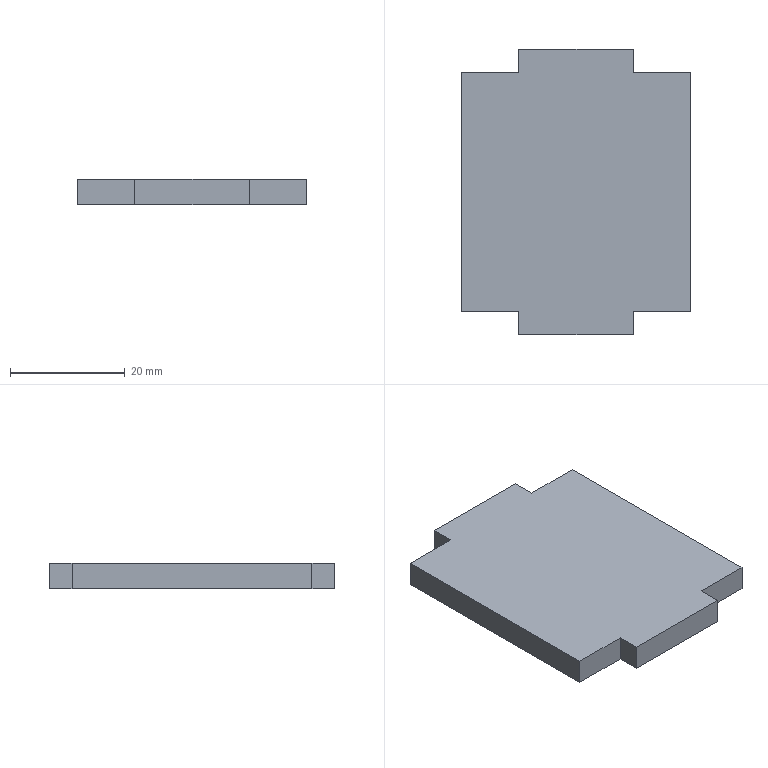Part | SolidWorks | features FlatPattern 1, SMBaseFlange 1, SheetMetal 1 | 1 solid | 14 faces | box 40 x 49.8 x 4.5 mm | volume 8244 mm3 | plane 14
STEP:
#1=CARTESIAN_POINT('',(58.167,-1154.371,0.));
#2=VERTEX_POINT('',#1);
#3=CARTESIAN_POINT('',(68.167,-1154.371,0.));
#4=VERTEX_POINT('',#3);
#5=CARTESIAN_POINT('',(68.167,-1154.371,0.));
#6=DIRECTION('',(1.,0.,0.));
#7=VECTOR('',#6,1000.);
#8=LINE('',#5,#7);
#9=EDGE_CURVE('',#2,#4,#8,.T.);
#10=ORIENTED_EDGE('',*,*,#9,.F.);
#11=CARTESIAN_POINT('',(58.167,-1154.371,-4.5));
#12=VERTEX_POINT('',#11);
#13=CARTESIAN_POINT('',(58.167,-1154.371,-4.5));
#14=DIRECTION('',(0.,0.,1.));
#15=VECTOR('',#14,1000.);
#16=LINE('',#13,#15);
#17=EDGE_CURVE('',#12,#2,#16,.T.);
#18=ORIENTED_EDGE('',*,*,#17,.F.);
#19=CARTESIAN_POINT('',(68.167,-1154.371,-4.5));
#20=VERTEX_POINT('',#19);
#21=CARTESIAN_POINT('',(68.167,-1154.371,-4.5));
#22=DIRECTION('',(1.,0.,0.));
#23=VECTOR('',#22,1000.);
#24=LINE('',#21,#23);
#25=EDGE_CURVE('',#12,#20,#24,.T.);
#26=ORIENTED_EDGE('',*,*,#25,.T.);
#27=CARTESIAN_POINT('',(68.167,-1154.371,-4.5));
#28=DIRECTION('',(0.,0.,1.));
#29=VECTOR('',#28,1000.);
#30=LINE('',#27,#29);
#31=EDGE_CURVE('',#20,#4,#30,.T.);
#32=ORIENTED_EDGE('',*,*,#31,.T.);
#33=EDGE_LOOP('',(#10,#18,#26,#32));
#34=FACE_OUTER_BOUND('',#33,.T.);
#35=CARTESIAN_POINT('',(68.167,-1154.371,-4.5));
#36=DIRECTION('',(0.,-1.,0.));
#37=DIRECTION('',(0.,0.,-1.));
#38=AXIS2_PLACEMENT_3D('',#35,#36,#37);
#39=PLANE('',#38);
#40=ADVANCED_FACE('',(#34),#39,.T.);
#41=CARTESIAN_POINT('',(58.167,-1158.371,0.));
#42=VERTEX_POINT('',#41);
#43=CARTESIAN_POINT('',(58.167,-1158.371,0.));
#44=DIRECTION('',(0.,1.,0.));
#45=VECTOR('',#44,1000.);
#46=LINE('',#43,#45);
#47=EDGE_CURVE('',#42,#2,#46,.T.);
#48=ORIENTED_EDGE('',*,*,#47,.F.);
#49=CARTESIAN_POINT('',(58.167,-1158.371,-4.5));
#50=VERTEX_POINT('',#49);
#51=CARTESIAN_POINT('',(58.167,-1158.371,-4.5));
#52=DIRECTION('',(0.,0.,1.));
#53=VECTOR('',#52,1000.);
#54=LINE('',#51,#53);
#55=EDGE_CURVE('',#50,#42,#54,.T.);
#56=ORIENTED_EDGE('',*,*,#55,.F.);
#57=CARTESIAN_POINT('',(58.167,-1158.371,-4.5));
#58=DIRECTION('',(0.,1.,0.));
#59=VECTOR('',#58,1000.);
#60=LINE('',#57,#59);
#61=EDGE_CURVE('',#50,#12,#60,.T.);
#62=ORIENTED_EDGE('',*,*,#61,.T.);
#63=ORIENTED_EDGE('',*,*,#17,.T.);
#64=EDGE_LOOP('',(#48,#56,#62,#63));
#65=FACE_OUTER_BOUND('',#64,.T.);
#66=CARTESIAN_POINT('',(58.167,-1158.371,-4.5));
#67=DIRECTION('',(1.,0.,0.));
#68=DIRECTION('',(0.,0.,-1.));
#69=AXIS2_PLACEMENT_3D('',#66,#67,#68);
#70=PLANE('',#69);
#71=ADVANCED_FACE('',(#65),#70,.T.);
#72=CARTESIAN_POINT('',(38.167,-1158.371,0.));
#73=VERTEX_POINT('',#72);
#74=CARTESIAN_POINT('',(38.167,-1158.371,0.));
#75=DIRECTION('',(1.,0.,0.));
#76=VECTOR('',#75,1000.);
#77=LINE('',#74,#76);
#78=EDGE_CURVE('',#73,#42,#77,.T.);
#79=ORIENTED_EDGE('',*,*,#78,.F.);
#80=CARTESIAN_POINT('',(38.167,-1158.371,-4.5));
#81=VERTEX_POINT('',#80);
#82=CARTESIAN_POINT('',(38.167,-1158.371,-4.5));
#83=DIRECTION('',(0.,0.,1.));
#84=VECTOR('',#83,1000.);
#85=LINE('',#82,#84);
#86=EDGE_CURVE('',#81,#73,#85,.T.);
#87=ORIENTED_EDGE('',*,*,#86,.F.);
#88=CARTESIAN_POINT('',(38.167,-1158.371,-4.5));
#89=DIRECTION('',(1.,0.,0.));
#90=VECTOR('',#89,1000.);
#91=LINE('',#88,#90);
#92=EDGE_CURVE('',#81,#50,#91,.T.);
#93=ORIENTED_EDGE('',*,*,#92,.T.);
#94=ORIENTED_EDGE('',*,*,#55,.T.);
#95=EDGE_LOOP('',(#79,#87,#93,#94));
#96=FACE_OUTER_BOUND('',#95,.T.);
#97=CARTESIAN_POINT('',(38.167,-1158.371,-4.5));
#98=DIRECTION('',(0.,-1.,0.));
#99=DIRECTION('',(0.,0.,-1.));
#100=AXIS2_PLACEMENT_3D('',#97,#98,#99);
#101=PLANE('',#100);
#102=ADVANCED_FACE('',(#96),#101,.T.);
#103=CARTESIAN_POINT('',(38.167,-1154.371,0.));
#104=VERTEX_POINT('',#103);
#105=CARTESIAN_POINT('',(38.167,-1158.371,0.));
#106=DIRECTION('',(0.,-1.,0.));
#107=VECTOR('',#106,1000.);
#108=LINE('',#105,#107);
#109=EDGE_CURVE('',#104,#73,#108,.T.);
#110=ORIENTED_EDGE('',*,*,#109,.F.);
#111=CARTESIAN_POINT('',(38.167,-1154.371,-4.5));
#112=VERTEX_POINT('',#111);
#113=CARTESIAN_POINT('',(38.167,-1154.371,-4.5));
#114=DIRECTION('',(0.,0.,1.));
#115=VECTOR('',#114,1000.);
#116=LINE('',#113,#115);
#117=EDGE_CURVE('',#112,#104,#116,.T.);
#118=ORIENTED_EDGE('',*,*,#117,.F.);
#119=CARTESIAN_POINT('',(38.167,-1158.371,-4.5));
#120=DIRECTION('',(0.,-1.,0.));
#121=VECTOR('',#120,1000.);
#122=LINE('',#119,#121);
#123=EDGE_CURVE('',#112,#81,#122,.T.);
#124=ORIENTED_EDGE('',*,*,#123,.T.);
#125=ORIENTED_EDGE('',*,*,#86,.T.);
#126=EDGE_LOOP('',(#110,#118,#124,#125));
#127=FACE_OUTER_BOUND('',#126,.T.);
#128=CARTESIAN_POINT('',(38.167,-1158.371,-4.5));
#129=DIRECTION('',(-1.,0.,0.));
#130=DIRECTION('',(0.,0.,1.));
#131=AXIS2_PLACEMENT_3D('',#128,#129,#130);
#132=PLANE('',#131);
#133=ADVANCED_FACE('',(#127),#132,.T.);
#134=CARTESIAN_POINT('',(28.167,-1154.371,0.));
#135=VERTEX_POINT('',#134);
#136=CARTESIAN_POINT('',(38.167,-1154.371,0.));
#137=DIRECTION('',(1.,0.,0.));
#138=VECTOR('',#137,1000.);
#139=LINE('',#136,#138);
#140=EDGE_CURVE('',#135,#104,#139,.T.);
#141=ORIENTED_EDGE('',*,*,#140,.F.);
#142=CARTESIAN_POINT('',(28.167,-1154.371,-4.5));
#143=VERTEX_POINT('',#142);
#144=CARTESIAN_POINT('',(28.167,-1154.371,-4.5));
#145=DIRECTION('',(0.,0.,1.));
#146=VECTOR('',#145,1000.);
#147=LINE('',#144,#146);
#148=EDGE_CURVE('',#143,#135,#147,.T.);
#149=ORIENTED_EDGE('',*,*,#148,.F.);
#150=CARTESIAN_POINT('',(38.167,-1154.371,-4.5));
#151=DIRECTION('',(1.,0.,0.));
#152=VECTOR('',#151,1000.);
#153=LINE('',#150,#152);
#154=EDGE_CURVE('',#143,#112,#153,.T.);
#155=ORIENTED_EDGE('',*,*,#154,.T.);
#156=ORIENTED_EDGE('',*,*,#117,.T.);
#157=EDGE_LOOP('',(#141,#149,#155,#156));
#158=FACE_OUTER_BOUND('',#157,.T.);
#159=CARTESIAN_POINT('',(38.167,-1154.371,-4.5));
#160=DIRECTION('',(0.,-1.,0.));
#161=DIRECTION('',(0.,0.,-1.));
#162=AXIS2_PLACEMENT_3D('',#159,#160,#161);
#163=PLANE('',#162);
#164=ADVANCED_FACE('',(#158),#163,.T.);
#165=CARTESIAN_POINT('',(28.167,-1112.571,0.));
#166=VERTEX_POINT('',#165);
#167=CARTESIAN_POINT('',(28.167,-1154.371,0.));
#168=DIRECTION('',(0.,-1.,0.));
#169=VECTOR('',#168,1000.);
#170=LINE('',#167,#169);
#171=EDGE_CURVE('',#166,#135,#170,.T.);
#172=ORIENTED_EDGE('',*,*,#171,.F.);
#173=CARTESIAN_POINT('',(28.167,-1112.571,-4.5));
#174=VERTEX_POINT('',#173);
#175=CARTESIAN_POINT('',(28.167,-1112.571,-4.5));
#176=DIRECTION('',(0.,0.,1.));
#177=VECTOR('',#176,1000.);
#178=LINE('',#175,#177);
#179=EDGE_CURVE('',#174,#166,#178,.T.);
#180=ORIENTED_EDGE('',*,*,#179,.F.);
#181=CARTESIAN_POINT('',(28.167,-1154.371,-4.5));
#182=DIRECTION('',(0.,-1.,0.));
#183=VECTOR('',#182,1000.);
#184=LINE('',#181,#183);
#185=EDGE_CURVE('',#174,#143,#184,.T.);
#186=ORIENTED_EDGE('',*,*,#185,.T.);
#187=ORIENTED_EDGE('',*,*,#148,.T.);
#188=EDGE_LOOP('',(#172,#180,#186,#187));
#189=FACE_OUTER_BOUND('',#188,.T.);
#190=CARTESIAN_POINT('',(28.167,-1154.371,-4.5));
#191=DIRECTION('',(-1.,0.,0.));
#192=DIRECTION('',(0.,0.,1.));
#193=AXIS2_PLACEMENT_3D('',#190,#191,#192);
#194=PLANE('',#193);
#195=ADVANCED_FACE('',(#189),#194,.T.);
#196=CARTESIAN_POINT('',(38.167,-1112.571,0.));
#197=VERTEX_POINT('',#196);
#198=CARTESIAN_POINT('',(28.167,-1112.571,0.));
#199=DIRECTION('',(-1.,0.,0.));
#200=VECTOR('',#199,1000.);
#201=LINE('',#198,#200);
#202=EDGE_CURVE('',#197,#166,#201,.T.);
#203=ORIENTED_EDGE('',*,*,#202,.F.);
#204=CARTESIAN_POINT('',(38.167,-1112.571,-4.5));
#205=VERTEX_POINT('',#204);
#206=CARTESIAN_POINT('',(38.167,-1112.571,-4.5));
#207=DIRECTION('',(0.,0.,1.));
#208=VECTOR('',#207,1000.);
#209=LINE('',#206,#208);
#210=EDGE_CURVE('',#205,#197,#209,.T.);
#211=ORIENTED_EDGE('',*,*,#210,.F.);
#212=CARTESIAN_POINT('',(28.167,-1112.571,-4.5));
#213=DIRECTION('',(-1.,0.,0.));
#214=VECTOR('',#213,1000.);
#215=LINE('',#212,#214);
#216=EDGE_CURVE('',#205,#174,#215,.T.);
#217=ORIENTED_EDGE('',*,*,#216,.T.);
#218=ORIENTED_EDGE('',*,*,#179,.T.);
#219=EDGE_LOOP('',(#203,#211,#217,#218));
#220=FACE_OUTER_BOUND('',#219,.T.);
#221=CARTESIAN_POINT('',(28.167,-1112.571,-4.5));
#222=DIRECTION('',(0.,1.,0.));
#223=DIRECTION('',(0.,0.,1.));
#224=AXIS2_PLACEMENT_3D('',#221,#222,#223);
#225=PLANE('',#224);
#226=ADVANCED_FACE('',(#220),#225,.T.);
#227=CARTESIAN_POINT('',(38.167,-1108.571,0.));
#228=VERTEX_POINT('',#227);
#229=CARTESIAN_POINT('',(38.167,-1108.571,0.));
#230=DIRECTION('',(0.,-1.,0.));
#231=VECTOR('',#230,1000.);
#232=LINE('',#229,#231);
#233=EDGE_CURVE('',#228,#197,#232,.T.);
#234=ORIENTED_EDGE('',*,*,#233,.F.);
#235=CARTESIAN_POINT('',(38.167,-1108.571,-4.5));
#236=VERTEX_POINT('',#235);
#237=CARTESIAN_POINT('',(38.167,-1108.571,-4.5));
#238=DIRECTION('',(0.,0.,1.));
#239=VECTOR('',#238,1000.);
#240=LINE('',#237,#239);
#241=EDGE_CURVE('',#236,#228,#240,.T.);
#242=ORIENTED_EDGE('',*,*,#241,.F.);
#243=CARTESIAN_POINT('',(38.167,-1108.571,-4.5));
#244=DIRECTION('',(0.,-1.,0.));
#245=VECTOR('',#244,1000.);
#246=LINE('',#243,#245);
#247=EDGE_CURVE('',#236,#205,#246,.T.);
#248=ORIENTED_EDGE('',*,*,#247,.T.);
#249=ORIENTED_EDGE('',*,*,#210,.T.);
#250=EDGE_LOOP('',(#234,#242,#248,#249));
#251=FACE_OUTER_BOUND('',#250,.T.);
#252=CARTESIAN_POINT('',(38.167,-1108.571,-4.5));
#253=DIRECTION('',(-1.,0.,0.));
#254=DIRECTION('',(0.,0.,1.));
#255=AXIS2_PLACEMENT_3D('',#252,#253,#254);
#256=PLANE('',#255);
#257=ADVANCED_FACE('',(#251),#256,.T.);
#258=CARTESIAN_POINT('',(58.167,-1108.571,0.));
#259=VERTEX_POINT('',#258);
#260=CARTESIAN_POINT('',(58.167,-1108.571,0.));
#261=DIRECTION('',(-1.,0.,0.));
#262=VECTOR('',#261,1000.);
#263=LINE('',#260,#262);
#264=EDGE_CURVE('',#259,#228,#263,.T.);
#265=ORIENTED_EDGE('',*,*,#264,.F.);
#266=CARTESIAN_POINT('',(58.167,-1108.571,-4.5));
#267=VERTEX_POINT('',#266);
#268=CARTESIAN_POINT('',(58.167,-1108.571,-4.5));
#269=DIRECTION('',(0.,0.,1.));
#270=VECTOR('',#269,1000.);
#271=LINE('',#268,#270);
#272=EDGE_CURVE('',#267,#259,#271,.T.);
#273=ORIENTED_EDGE('',*,*,#272,.F.);
#274=CARTESIAN_POINT('',(58.167,-1108.571,-4.5));
#275=DIRECTION('',(-1.,0.,0.));
#276=VECTOR('',#275,1000.);
#277=LINE('',#274,#276);
#278=EDGE_CURVE('',#267,#236,#277,.T.);
#279=ORIENTED_EDGE('',*,*,#278,.T.);
#280=ORIENTED_EDGE('',*,*,#241,.T.);
#281=EDGE_LOOP('',(#265,#273,#279,#280));
#282=FACE_OUTER_BOUND('',#281,.T.);
#283=CARTESIAN_POINT('',(58.167,-1108.571,-4.5));
#284=DIRECTION('',(0.,1.,0.));
#285=DIRECTION('',(0.,0.,1.));
#286=AXIS2_PLACEMENT_3D('',#283,#284,#285);
#287=PLANE('',#286);
#288=ADVANCED_FACE('',(#282),#287,.T.);
#289=CARTESIAN_POINT('',(58.167,-1112.571,0.));
#290=VERTEX_POINT('',#289);
#291=CARTESIAN_POINT('',(58.167,-1112.571,0.));
#292=DIRECTION('',(0.,1.,0.));
#293=VECTOR('',#292,1000.);
#294=LINE('',#291,#293);
#295=EDGE_CURVE('',#290,#259,#294,.T.);
#296=ORIENTED_EDGE('',*,*,#295,.F.);
#297=CARTESIAN_POINT('',(58.167,-1112.571,-4.5));
#298=VERTEX_POINT('',#297);
#299=CARTESIAN_POINT('',(58.167,-1112.571,-4.5));
#300=DIRECTION('',(0.,0.,1.));
#301=VECTOR('',#300,1000.);
#302=LINE('',#299,#301);
#303=EDGE_CURVE('',#298,#290,#302,.T.);
#304=ORIENTED_EDGE('',*,*,#303,.F.);
#305=CARTESIAN_POINT('',(58.167,-1112.571,-4.5));
#306=DIRECTION('',(0.,1.,0.));
#307=VECTOR('',#306,1000.);
#308=LINE('',#305,#307);
#309=EDGE_CURVE('',#298,#267,#308,.T.);
#310=ORIENTED_EDGE('',*,*,#309,.T.);
#311=ORIENTED_EDGE('',*,*,#272,.T.);
#312=EDGE_LOOP('',(#296,#304,#310,#311));
#313=FACE_OUTER_BOUND('',#312,.T.);
#314=CARTESIAN_POINT('',(58.167,-1112.571,-4.5));
#315=DIRECTION('',(1.,0.,0.));
#316=DIRECTION('',(0.,0.,-1.));
#317=AXIS2_PLACEMENT_3D('',#314,#315,#316);
#318=PLANE('',#317);
#319=ADVANCED_FACE('',(#313),#318,.T.);
#320=CARTESIAN_POINT('',(68.167,-1112.571,0.));
#321=VERTEX_POINT('',#320);
#322=CARTESIAN_POINT('',(58.167,-1112.571,0.));
#323=DIRECTION('',(-1.,0.,0.));
#324=VECTOR('',#323,1000.);
#325=LINE('',#322,#324);
#326=EDGE_CURVE('',#321,#290,#325,.T.);
#327=ORIENTED_EDGE('',*,*,#326,.F.);
#328=CARTESIAN_POINT('',(68.167,-1112.571,-4.5));
#329=VERTEX_POINT('',#328);
#330=CARTESIAN_POINT('',(68.167,-1112.571,-4.5));
#331=DIRECTION('',(0.,0.,1.));
#332=VECTOR('',#331,1000.);
#333=LINE('',#330,#332);
#334=EDGE_CURVE('',#329,#321,#333,.T.);
#335=ORIENTED_EDGE('',*,*,#334,.F.);
#336=CARTESIAN_POINT('',(58.167,-1112.571,-4.5));
#337=DIRECTION('',(-1.,0.,0.));
#338=VECTOR('',#337,1000.);
#339=LINE('',#336,#338);
#340=EDGE_CURVE('',#329,#298,#339,.T.);
#341=ORIENTED_EDGE('',*,*,#340,.T.);
#342=ORIENTED_EDGE('',*,*,#303,.T.);
#343=EDGE_LOOP('',(#327,#335,#341,#342));
#344=FACE_OUTER_BOUND('',#343,.T.);
#345=CARTESIAN_POINT('',(58.167,-1112.571,-4.5));
#346=DIRECTION('',(0.,1.,0.));
#347=DIRECTION('',(0.,0.,1.));
#348=AXIS2_PLACEMENT_3D('',#345,#346,#347);
#349=PLANE('',#348);
#350=ADVANCED_FACE('',(#344),#349,.T.);
#351=CARTESIAN_POINT('',(68.167,-1154.371,0.));
#352=DIRECTION('',(0.,1.,0.));
#353=VECTOR('',#352,1000.);
#354=LINE('',#351,#353);
#355=EDGE_CURVE('',#4,#321,#354,.T.);
#356=ORIENTED_EDGE('',*,*,#355,.F.);
#357=ORIENTED_EDGE('',*,*,#31,.F.);
#358=CARTESIAN_POINT('',(68.167,-1154.371,-4.5));
#359=DIRECTION('',(0.,1.,0.));
#360=VECTOR('',#359,1000.);
#361=LINE('',#358,#360);
#362=EDGE_CURVE('',#20,#329,#361,.T.);
#363=ORIENTED_EDGE('',*,*,#362,.T.);
#364=ORIENTED_EDGE('',*,*,#334,.T.);
#365=EDGE_LOOP('',(#356,#357,#363,#364));
#366=FACE_OUTER_BOUND('',#365,.T.);
#367=CARTESIAN_POINT('',(68.167,-1154.371,-4.5));
#368=DIRECTION('',(1.,0.,0.));
#369=DIRECTION('',(0.,1.,0.));
#370=AXIS2_PLACEMENT_3D('',#367,#368,#369);
#371=PLANE('',#370);
#372=ADVANCED_FACE('',(#366),#371,.T.);
#373=ORIENTED_EDGE('',*,*,#25,.F.);
#374=ORIENTED_EDGE('',*,*,#61,.F.);
#375=ORIENTED_EDGE('',*,*,#92,.F.);
#376=ORIENTED_EDGE('',*,*,#123,.F.);
#377=ORIENTED_EDGE('',*,*,#154,.F.);
#378=ORIENTED_EDGE('',*,*,#185,.F.);
#379=ORIENTED_EDGE('',*,*,#216,.F.);
#380=ORIENTED_EDGE('',*,*,#247,.F.);
#381=ORIENTED_EDGE('',*,*,#278,.F.);
#382=ORIENTED_EDGE('',*,*,#309,.F.);
#383=ORIENTED_EDGE('',*,*,#340,.F.);
#384=ORIENTED_EDGE('',*,*,#362,.F.);
#385=EDGE_LOOP('',(#373,#374,#375,#376,#377,#378,#379,#380,#381,#382,#383,#384));
#386=FACE_OUTER_BOUND('',#385,.T.);
#387=CARTESIAN_POINT('',(0.,0.,-4.5));
#388=DIRECTION('',(0.,0.,-1.));
#389=DIRECTION('',(-1.,0.,0.));
#390=AXIS2_PLACEMENT_3D('',#387,#388,#389);
#391=PLANE('',#390);
#392=ADVANCED_FACE('',(#386),#391,.T.);
#393=ORIENTED_EDGE('',*,*,#9,.T.);
#394=ORIENTED_EDGE('',*,*,#355,.T.);
#395=ORIENTED_EDGE('',*,*,#326,.T.);
#396=ORIENTED_EDGE('',*,*,#295,.T.);
#397=ORIENTED_EDGE('',*,*,#264,.T.);
#398=ORIENTED_EDGE('',*,*,#233,.T.);
#399=ORIENTED_EDGE('',*,*,#202,.T.);
#400=ORIENTED_EDGE('',*,*,#171,.T.);
#401=ORIENTED_EDGE('',*,*,#140,.T.);
#402=ORIENTED_EDGE('',*,*,#109,.T.);
#403=ORIENTED_EDGE('',*,*,#78,.T.);
#404=ORIENTED_EDGE('',*,*,#47,.T.);
#405=EDGE_LOOP('',(#393,#394,#395,#396,#397,#398,#399,#400,#401,#402,#403,#404));
#406=FACE_OUTER_BOUND('',#405,.T.);
#407=CARTESIAN_POINT('',(0.,0.,0.));
#408=DIRECTION('',(0.,0.,-1.));
#409=DIRECTION('',(-1.,0.,0.));
#410=AXIS2_PLACEMENT_3D('',#407,#408,#409);
#411=PLANE('',#410);
#412=ADVANCED_FACE('',(#406),#411,.F.);
#413=CLOSED_SHELL('',(#40,#71,#102,#133,#164,#195,#226,#257,#288,#319,#350,#372,#392,#412));
#414=MANIFOLD_SOLID_BREP('',#413);
#415=CARTESIAN_POINT('',(0.,0.,0.));
#416=DIRECTION('',(0.,0.,1.));
#417=DIRECTION('',(1.,0.,0.));
#418=AXIS2_PLACEMENT_3D('',#415,#416,#417);
#419=(LENGTH_UNIT()NAMED_UNIT(*)SI_UNIT(.MILLI.,.METRE.));
#420=UNCERTAINTY_MEASURE_WITH_UNIT(LENGTH_MEASURE(0.00001),#419,'','');
#421=(NAMED_UNIT(*)PLANE_ANGLE_UNIT()SI_UNIT($,.RADIAN.));
#422=(NAMED_UNIT(*)SI_UNIT($,.STERADIAN.)SOLID_ANGLE_UNIT());
#423=(GEOMETRIC_REPRESENTATION_CONTEXT(3)GLOBAL_UNCERTAINTY_ASSIGNED_CONTEXT((#420))GLOBAL_UNIT_ASSIGNED_CONTEXT((#419,#421,#422))REPRESENTATION_CONTEXT('',''));
#424=ADVANCED_BREP_SHAPE_REPRESENTATION('',(#414,#418),#423);